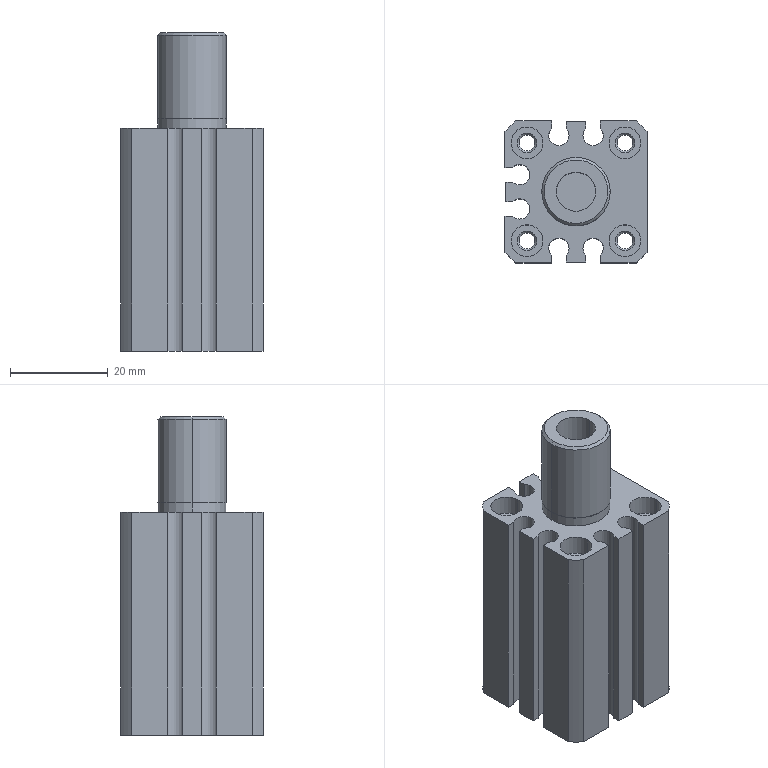Part | STEP file | 1 solid | 144 faces | box 29 x 29 x 65 mm | volume 26524 mm3 | cylinder 64 | plane 52 | cone 28 | commonest cylinder face diameters 3.242 x18 6.5 x16 3.5 x8 4.15 x6 4.134 x4 38 x4